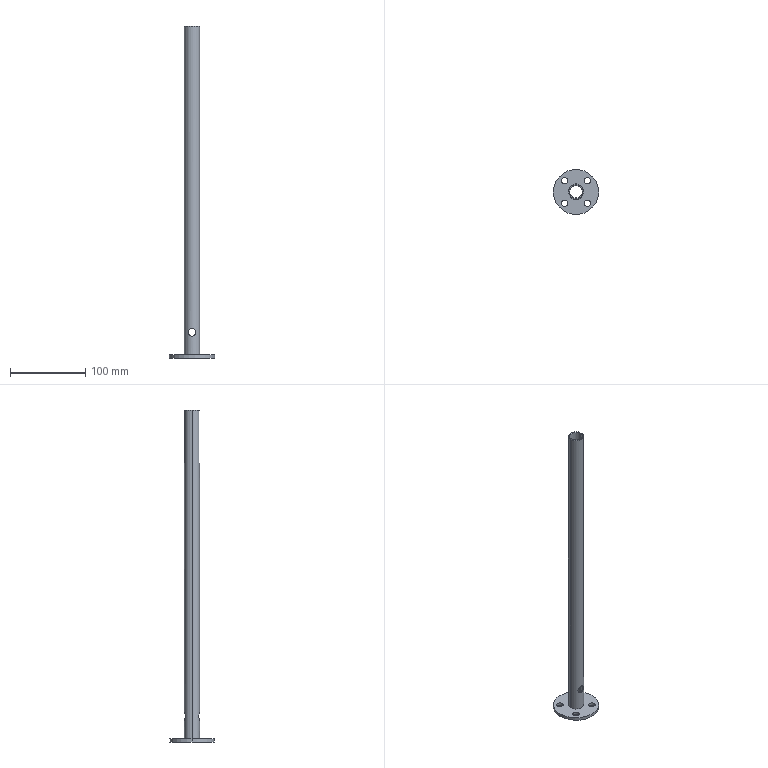Part | STEP file | Switch support rod_default<machined> | 2 solids | 28 faces | box 60 x 60 x 440 mm | volume 47255 mm3 | cylinder 20 | plane 4 | cone 4 | commonest cylinder face diameters 8.5 x8 10 x4 20 x4 17 x2 60 x2